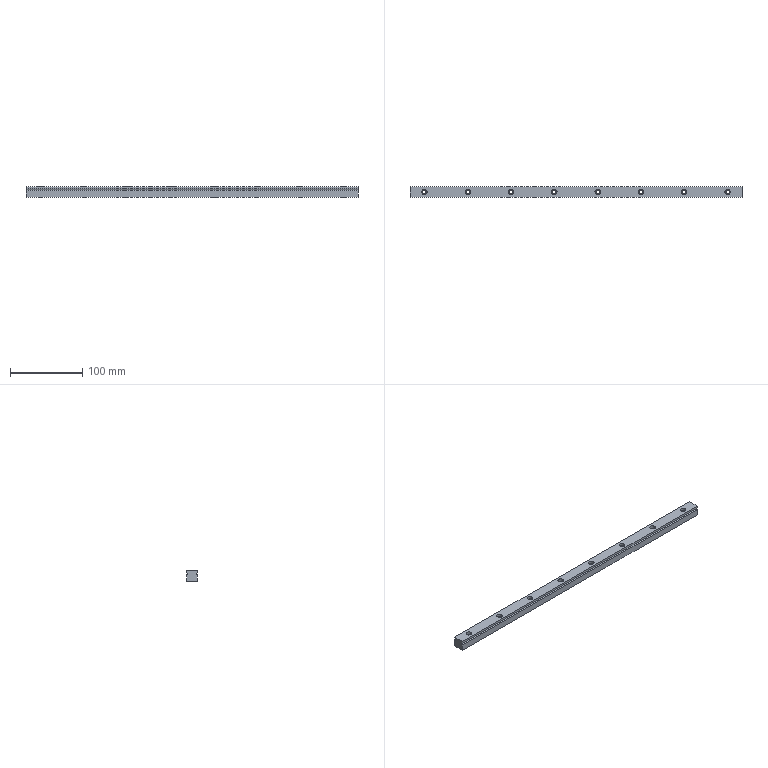Part | SolidWorks | features BaseBody 1 | 1 solid | 50 faces | box 460 x 15 x 15 mm | volume 98244 mm3 | cylinder 34 | plane 16 | commonest cylinder face diameters 4.5 x16 7.5 x16 2.6 x2
STEP:
#1=CARTESIAN_POINT('',(212.25,0.,0.));
#2=VERTEX_POINT('',#1);
#3=CARTESIAN_POINT('',(207.75,0.,0.));
#4=VERTEX_POINT('',#3);
#5=CARTESIAN_POINT('',(210.,0.,0.));
#6=DIRECTION('',(0.,0.,-1.));
#7=DIRECTION('',(1.,0.,0.));
#8=AXIS2_PLACEMENT_3D('',#5,#6,#7);
#9=CIRCLE('',#8,2.25);
#10=EDGE_CURVE('',#2,#4,#9,.T.);
#11=ORIENTED_EDGE('',*,*,#10,.T.);
#12=CARTESIAN_POINT('',(207.75,0.,11.));
#13=VERTEX_POINT('',#12);
#14=CARTESIAN_POINT('',(207.75,0.,-1.));
#15=DIRECTION('',(0.,0.,1.));
#16=VECTOR('',#15,1000.);
#17=LINE('',#14,#16);
#18=EDGE_CURVE('',#4,#13,#17,.T.);
#19=ORIENTED_EDGE('',*,*,#18,.T.);
#20=CARTESIAN_POINT('',(212.25,0.,11.));
#21=VERTEX_POINT('',#20);
#22=CARTESIAN_POINT('',(210.,0.,11.));
#23=DIRECTION('',(0.,0.,-1.));
#24=DIRECTION('',(1.,0.,0.));
#25=AXIS2_PLACEMENT_3D('',#22,#23,#24);
#26=CIRCLE('',#25,2.25);
#27=EDGE_CURVE('',#21,#13,#26,.T.);
#28=ORIENTED_EDGE('',*,*,#27,.F.);
#29=CARTESIAN_POINT('',(212.25,0.,-1.));
#30=DIRECTION('',(0.,0.,1.));
#31=VECTOR('',#30,1000.);
#32=LINE('',#29,#31);
#33=EDGE_CURVE('',#2,#21,#32,.T.);
#34=ORIENTED_EDGE('',*,*,#33,.F.);
#35=EDGE_LOOP('',(#11,#19,#28,#34));
#36=FACE_OUTER_BOUND('',#35,.T.);
#37=CARTESIAN_POINT('',(210.,0.,-1.));
#38=DIRECTION('',(0.,0.,1.));
#39=DIRECTION('',(1.,0.,0.));
#40=AXIS2_PLACEMENT_3D('',#37,#38,#39);
#41=CYLINDRICAL_SURFACE('',#40,2.25);
#42=ADVANCED_FACE('',(#36),#41,.F.);
#43=CARTESIAN_POINT('',(152.25,0.,0.));
#44=VERTEX_POINT('',#43);
#45=CARTESIAN_POINT('',(147.75,0.,0.));
#46=VERTEX_POINT('',#45);
#47=CARTESIAN_POINT('',(150.,0.,0.));
#48=DIRECTION('',(0.,0.,-1.));
#49=DIRECTION('',(1.,0.,0.));
#50=AXIS2_PLACEMENT_3D('',#47,#48,#49);
#51=CIRCLE('',#50,2.25);
#52=EDGE_CURVE('',#44,#46,#51,.T.);
#53=ORIENTED_EDGE('',*,*,#52,.T.);
#54=CARTESIAN_POINT('',(147.75,0.,11.));
#55=VERTEX_POINT('',#54);
#56=CARTESIAN_POINT('',(147.75,0.,-1.));
#57=DIRECTION('',(0.,0.,1.));
#58=VECTOR('',#57,1000.);
#59=LINE('',#56,#58);
#60=EDGE_CURVE('',#46,#55,#59,.T.);
#61=ORIENTED_EDGE('',*,*,#60,.T.);
#62=CARTESIAN_POINT('',(152.25,0.,11.));
#63=VERTEX_POINT('',#62);
#64=CARTESIAN_POINT('',(150.,0.,11.));
#65=DIRECTION('',(0.,0.,-1.));
#66=DIRECTION('',(1.,0.,0.));
#67=AXIS2_PLACEMENT_3D('',#64,#65,#66);
#68=CIRCLE('',#67,2.25);
#69=EDGE_CURVE('',#63,#55,#68,.T.);
#70=ORIENTED_EDGE('',*,*,#69,.F.);
#71=CARTESIAN_POINT('',(152.25,0.,-1.));
#72=DIRECTION('',(0.,0.,1.));
#73=VECTOR('',#72,1000.);
#74=LINE('',#71,#73);
#75=EDGE_CURVE('',#44,#63,#74,.T.);
#76=ORIENTED_EDGE('',*,*,#75,.F.);
#77=EDGE_LOOP('',(#53,#61,#70,#76));
#78=FACE_OUTER_BOUND('',#77,.T.);
#79=CARTESIAN_POINT('',(150.,0.,-1.));
#80=DIRECTION('',(0.,0.,1.));
#81=DIRECTION('',(1.,0.,0.));
#82=AXIS2_PLACEMENT_3D('',#79,#80,#81);
#83=CYLINDRICAL_SURFACE('',#82,2.25);
#84=ADVANCED_FACE('',(#78),#83,.F.);
#85=CARTESIAN_POINT('',(92.25,0.,0.));
#86=VERTEX_POINT('',#85);
#87=CARTESIAN_POINT('',(87.75,0.,0.));
#88=VERTEX_POINT('',#87);
#89=CARTESIAN_POINT('',(90.,0.,0.));
#90=DIRECTION('',(0.,0.,-1.));
#91=DIRECTION('',(1.,0.,0.));
#92=AXIS2_PLACEMENT_3D('',#89,#90,#91);
#93=CIRCLE('',#92,2.25);
#94=EDGE_CURVE('',#86,#88,#93,.T.);
#95=ORIENTED_EDGE('',*,*,#94,.T.);
#96=CARTESIAN_POINT('',(87.75,0.,11.));
#97=VERTEX_POINT('',#96);
#98=CARTESIAN_POINT('',(87.75,0.,-1.));
#99=DIRECTION('',(0.,0.,1.));
#100=VECTOR('',#99,1000.);
#101=LINE('',#98,#100);
#102=EDGE_CURVE('',#88,#97,#101,.T.);
#103=ORIENTED_EDGE('',*,*,#102,.T.);
#104=CARTESIAN_POINT('',(92.25,0.,11.));
#105=VERTEX_POINT('',#104);
#106=CARTESIAN_POINT('',(90.,0.,11.));
#107=DIRECTION('',(0.,0.,-1.));
#108=DIRECTION('',(1.,0.,0.));
#109=AXIS2_PLACEMENT_3D('',#106,#107,#108);
#110=CIRCLE('',#109,2.25);
#111=EDGE_CURVE('',#105,#97,#110,.T.);
#112=ORIENTED_EDGE('',*,*,#111,.F.);
#113=CARTESIAN_POINT('',(92.25,0.,-1.));
#114=DIRECTION('',(0.,0.,1.));
#115=VECTOR('',#114,1000.);
#116=LINE('',#113,#115);
#117=EDGE_CURVE('',#86,#105,#116,.T.);
#118=ORIENTED_EDGE('',*,*,#117,.F.);
#119=EDGE_LOOP('',(#95,#103,#112,#118));
#120=FACE_OUTER_BOUND('',#119,.T.);
#121=CARTESIAN_POINT('',(90.,0.,-1.));
#122=DIRECTION('',(0.,0.,1.));
#123=DIRECTION('',(1.,0.,0.));
#124=AXIS2_PLACEMENT_3D('',#121,#122,#123);
#125=CYLINDRICAL_SURFACE('',#124,2.25);
#126=ADVANCED_FACE('',(#120),#125,.F.);
#127=CARTESIAN_POINT('',(32.25,0.,0.));
#128=VERTEX_POINT('',#127);
#129=CARTESIAN_POINT('',(27.75,0.,0.));
#130=VERTEX_POINT('',#129);
#131=CARTESIAN_POINT('',(30.,0.,0.));
#132=DIRECTION('',(0.,0.,-1.));
#133=DIRECTION('',(1.,0.,0.));
#134=AXIS2_PLACEMENT_3D('',#131,#132,#133);
#135=CIRCLE('',#134,2.25);
#136=EDGE_CURVE('',#128,#130,#135,.T.);
#137=ORIENTED_EDGE('',*,*,#136,.T.);
#138=CARTESIAN_POINT('',(27.75,0.,11.));
#139=VERTEX_POINT('',#138);
#140=CARTESIAN_POINT('',(27.75,0.,-1.));
#141=DIRECTION('',(0.,0.,1.));
#142=VECTOR('',#141,1000.);
#143=LINE('',#140,#142);
#144=EDGE_CURVE('',#130,#139,#143,.T.);
#145=ORIENTED_EDGE('',*,*,#144,.T.);
#146=CARTESIAN_POINT('',(32.25,0.,11.));
#147=VERTEX_POINT('',#146);
#148=CARTESIAN_POINT('',(30.,0.,11.));
#149=DIRECTION('',(0.,0.,-1.));
#150=DIRECTION('',(1.,0.,0.));
#151=AXIS2_PLACEMENT_3D('',#148,#149,#150);
#152=CIRCLE('',#151,2.25);
#153=EDGE_CURVE('',#147,#139,#152,.T.);
#154=ORIENTED_EDGE('',*,*,#153,.F.);
#155=CARTESIAN_POINT('',(32.25,0.,-1.));
#156=DIRECTION('',(0.,0.,1.));
#157=VECTOR('',#156,1000.);
#158=LINE('',#155,#157);
#159=EDGE_CURVE('',#128,#147,#158,.T.);
#160=ORIENTED_EDGE('',*,*,#159,.F.);
#161=EDGE_LOOP('',(#137,#145,#154,#160));
#162=FACE_OUTER_BOUND('',#161,.T.);
#163=CARTESIAN_POINT('',(30.,0.,-1.));
#164=DIRECTION('',(0.,0.,1.));
#165=DIRECTION('',(1.,0.,0.));
#166=AXIS2_PLACEMENT_3D('',#163,#164,#165);
#167=CYLINDRICAL_SURFACE('',#166,2.25);
#168=ADVANCED_FACE('',(#162),#167,.F.);
#169=CARTESIAN_POINT('',(-27.75,0.,0.));
#170=VERTEX_POINT('',#169);
#171=CARTESIAN_POINT('',(-32.25,0.,0.));
#172=VERTEX_POINT('',#171);
#173=CARTESIAN_POINT('',(-30.,0.,0.));
#174=DIRECTION('',(0.,0.,-1.));
#175=DIRECTION('',(1.,0.,0.));
#176=AXIS2_PLACEMENT_3D('',#173,#174,#175);
#177=CIRCLE('',#176,2.25);
#178=EDGE_CURVE('',#170,#172,#177,.T.);
#179=ORIENTED_EDGE('',*,*,#178,.T.);
#180=CARTESIAN_POINT('',(-32.25,0.,11.));
#181=VERTEX_POINT('',#180);
#182=CARTESIAN_POINT('',(-32.25,0.,-1.));
#183=DIRECTION('',(0.,0.,1.));
#184=VECTOR('',#183,1000.);
#185=LINE('',#182,#184);
#186=EDGE_CURVE('',#172,#181,#185,.T.);
#187=ORIENTED_EDGE('',*,*,#186,.T.);
#188=CARTESIAN_POINT('',(-27.75,0.,11.));
#189=VERTEX_POINT('',#188);
#190=CARTESIAN_POINT('',(-30.,0.,11.));
#191=DIRECTION('',(0.,0.,-1.));
#192=DIRECTION('',(1.,0.,0.));
#193=AXIS2_PLACEMENT_3D('',#190,#191,#192);
#194=CIRCLE('',#193,2.25);
#195=EDGE_CURVE('',#189,#181,#194,.T.);
#196=ORIENTED_EDGE('',*,*,#195,.F.);
#197=CARTESIAN_POINT('',(-27.75,0.,-1.));
#198=DIRECTION('',(0.,0.,1.));
#199=VECTOR('',#198,1000.);
#200=LINE('',#197,#199);
#201=EDGE_CURVE('',#170,#189,#200,.T.);
#202=ORIENTED_EDGE('',*,*,#201,.F.);
#203=EDGE_LOOP('',(#179,#187,#196,#202));
#204=FACE_OUTER_BOUND('',#203,.T.);
#205=CARTESIAN_POINT('',(-30.,0.,-1.));
#206=DIRECTION('',(0.,0.,1.));
#207=DIRECTION('',(1.,0.,0.));
#208=AXIS2_PLACEMENT_3D('',#205,#206,#207);
#209=CYLINDRICAL_SURFACE('',#208,2.25);
#210=ADVANCED_FACE('',(#204),#209,.F.);
#211=CARTESIAN_POINT('',(-87.75,0.,0.));
#212=VERTEX_POINT('',#211);
#213=CARTESIAN_POINT('',(-92.25,0.,0.));
#214=VERTEX_POINT('',#213);
#215=CARTESIAN_POINT('',(-90.,0.,0.));
#216=DIRECTION('',(0.,0.,-1.));
#217=DIRECTION('',(1.,0.,0.));
#218=AXIS2_PLACEMENT_3D('',#215,#216,#217);
#219=CIRCLE('',#218,2.25);
#220=EDGE_CURVE('',#212,#214,#219,.T.);
#221=ORIENTED_EDGE('',*,*,#220,.T.);
#222=CARTESIAN_POINT('',(-92.25,0.,11.));
#223=VERTEX_POINT('',#222);
#224=CARTESIAN_POINT('',(-92.25,0.,-1.));
#225=DIRECTION('',(0.,0.,1.));
#226=VECTOR('',#225,1000.);
#227=LINE('',#224,#226);
#228=EDGE_CURVE('',#214,#223,#227,.T.);
#229=ORIENTED_EDGE('',*,*,#228,.T.);
#230=CARTESIAN_POINT('',(-87.75,0.,11.));
#231=VERTEX_POINT('',#230);
#232=CARTESIAN_POINT('',(-90.,0.,11.));
#233=DIRECTION('',(0.,0.,-1.));
#234=DIRECTION('',(1.,0.,0.));
#235=AXIS2_PLACEMENT_3D('',#232,#233,#234);
#236=CIRCLE('',#235,2.25);
#237=EDGE_CURVE('',#231,#223,#236,.T.);
#238=ORIENTED_EDGE('',*,*,#237,.F.);
#239=CARTESIAN_POINT('',(-87.75,0.,-1.));
#240=DIRECTION('',(0.,0.,1.));
#241=VECTOR('',#240,1000.);
#242=LINE('',#239,#241);
#243=EDGE_CURVE('',#212,#231,#242,.T.);
#244=ORIENTED_EDGE('',*,*,#243,.F.);
#245=EDGE_LOOP('',(#221,#229,#238,#244));
#246=FACE_OUTER_BOUND('',#245,.T.);
#247=CARTESIAN_POINT('',(-90.,0.,-1.));
#248=DIRECTION('',(0.,0.,1.));
#249=DIRECTION('',(1.,0.,0.));
#250=AXIS2_PLACEMENT_3D('',#247,#248,#249);
#251=CYLINDRICAL_SURFACE('',#250,2.25);
#252=ADVANCED_FACE('',(#246),#251,.F.);
#253=CARTESIAN_POINT('',(-147.75,0.,0.));
#254=VERTEX_POINT('',#253);
#255=CARTESIAN_POINT('',(-152.25,0.,0.));
#256=VERTEX_POINT('',#255);
#257=CARTESIAN_POINT('',(-150.,0.,0.));
#258=DIRECTION('',(0.,0.,-1.));
#259=DIRECTION('',(1.,0.,0.));
#260=AXIS2_PLACEMENT_3D('',#257,#258,#259);
#261=CIRCLE('',#260,2.25);
#262=EDGE_CURVE('',#254,#256,#261,.T.);
#263=ORIENTED_EDGE('',*,*,#262,.T.);
#264=CARTESIAN_POINT('',(-152.25,0.,11.));
#265=VERTEX_POINT('',#264);
#266=CARTESIAN_POINT('',(-152.25,0.,-1.));
#267=DIRECTION('',(0.,0.,1.));
#268=VECTOR('',#267,1000.);
#269=LINE('',#266,#268);
#270=EDGE_CURVE('',#256,#265,#269,.T.);
#271=ORIENTED_EDGE('',*,*,#270,.T.);
#272=CARTESIAN_POINT('',(-147.75,0.,11.));
#273=VERTEX_POINT('',#272);
#274=CARTESIAN_POINT('',(-150.,0.,11.));
#275=DIRECTION('',(0.,0.,-1.));
#276=DIRECTION('',(1.,0.,0.));
#277=AXIS2_PLACEMENT_3D('',#274,#275,#276);
#278=CIRCLE('',#277,2.25);
#279=EDGE_CURVE('',#273,#265,#278,.T.);
#280=ORIENTED_EDGE('',*,*,#279,.F.);
#281=CARTESIAN_POINT('',(-147.75,0.,-1.));
#282=DIRECTION('',(0.,0.,1.));
#283=VECTOR('',#282,1000.);
#284=LINE('',#281,#283);
#285=EDGE_CURVE('',#254,#273,#284,.T.);
#286=ORIENTED_EDGE('',*,*,#285,.F.);
#287=EDGE_LOOP('',(#263,#271,#280,#286));
#288=FACE_OUTER_BOUND('',#287,.T.);
#289=CARTESIAN_POINT('',(-150.,0.,-1.));
#290=DIRECTION('',(0.,0.,1.));
#291=DIRECTION('',(1.,0.,0.));
#292=AXIS2_PLACEMENT_3D('',#289,#290,#291);
#293=CYLINDRICAL_SURFACE('',#292,2.25);
#294=ADVANCED_FACE('',(#288),#293,.F.);
#295=CARTESIAN_POINT('',(-207.75,0.,0.));
#296=VERTEX_POINT('',#295);
#297=CARTESIAN_POINT('',(-212.25,0.,0.));
#298=VERTEX_POINT('',#297);
#299=CARTESIAN_POINT('',(-210.,0.,0.));
#300=DIRECTION('',(0.,0.,-1.));
#301=DIRECTION('',(1.,0.,0.));
#302=AXIS2_PLACEMENT_3D('',#299,#300,#301);
#303=CIRCLE('',#302,2.25);
#304=EDGE_CURVE('',#296,#298,#303,.T.);
#305=ORIENTED_EDGE('',*,*,#304,.T.);
#306=CARTESIAN_POINT('',(-212.25,0.,11.));
#307=VERTEX_POINT('',#306);
#308=CARTESIAN_POINT('',(-212.25,0.,-1.));
#309=DIRECTION('',(0.,0.,1.));
#310=VECTOR('',#309,1000.);
#311=LINE('',#308,#310);
#312=EDGE_CURVE('',#298,#307,#311,.T.);
#313=ORIENTED_EDGE('',*,*,#312,.T.);
#314=CARTESIAN_POINT('',(-207.75,0.,11.));
#315=VERTEX_POINT('',#314);
#316=CARTESIAN_POINT('',(-210.,0.,11.));
#317=DIRECTION('',(0.,0.,-1.));
#318=DIRECTION('',(1.,0.,0.));
#319=AXIS2_PLACEMENT_3D('',#316,#317,#318);
#320=CIRCLE('',#319,2.25);
#321=EDGE_CURVE('',#315,#307,#320,.T.);
#322=ORIENTED_EDGE('',*,*,#321,.F.);
#323=CARTESIAN_POINT('',(-207.75,0.,-1.));
#324=DIRECTION('',(0.,0.,1.));
#325=VECTOR('',#324,1000.);
#326=LINE('',#323,#325);
#327=EDGE_CURVE('',#296,#315,#326,.T.);
#328=ORIENTED_EDGE('',*,*,#327,.F.);
#329=EDGE_LOOP('',(#305,#313,#322,#328));
#330=FACE_OUTER_BOUND('',#329,.T.);
#331=CARTESIAN_POINT('',(-210.,0.,-1.));
#332=DIRECTION('',(0.,0.,1.));
#333=DIRECTION('',(1.,0.,0.));
#334=AXIS2_PLACEMENT_3D('',#331,#332,#333);
#335=CYLINDRICAL_SURFACE('',#334,2.25);
#336=ADVANCED_FACE('',(#330),#335,.F.);
#337=CARTESIAN_POINT('',(206.25,0.,11.));
#338=VERTEX_POINT('',#337);
#339=CARTESIAN_POINT('',(213.75,0.,11.));
#340=VERTEX_POINT('',#339);
#341=CARTESIAN_POINT('',(210.,0.,11.));
#342=DIRECTION('',(0.,0.,1.));
#343=DIRECTION('',(1.,0.,0.));
#344=AXIS2_PLACEMENT_3D('',#341,#342,#343);
#345=CIRCLE('',#344,3.75);
#346=EDGE_CURVE('',#338,#340,#345,.T.);
#347=ORIENTED_EDGE('',*,*,#346,.F.);
#348=CARTESIAN_POINT('',(206.25,0.,15.));
#349=VERTEX_POINT('',#348);
#350=CARTESIAN_POINT('',(206.25,0.,11.));
#351=DIRECTION('',(0.,0.,1.));
#352=VECTOR('',#351,1000.);
#353=LINE('',#350,#352);
#354=EDGE_CURVE('',#338,#349,#353,.T.);
#355=ORIENTED_EDGE('',*,*,#354,.T.);
#356=CARTESIAN_POINT('',(213.75,0.,15.));
#357=VERTEX_POINT('',#356);
#358=CARTESIAN_POINT('',(210.,0.,15.));
#359=DIRECTION('',(0.,0.,-1.));
#360=DIRECTION('',(1.,0.,0.));
#361=AXIS2_PLACEMENT_3D('',#358,#359,#360);
#362=CIRCLE('',#361,3.75);
#363=EDGE_CURVE('',#357,#349,#362,.T.);
#364=ORIENTED_EDGE('',*,*,#363,.F.);
#365=CARTESIAN_POINT('',(213.75,0.,11.));
#366=DIRECTION('',(0.,0.,1.));
#367=VECTOR('',#366,1000.);
#368=LINE('',#365,#367);
#369=EDGE_CURVE('',#340,#357,#368,.T.);
#370=ORIENTED_EDGE('',*,*,#369,.F.);
#371=EDGE_LOOP('',(#347,#355,#364,#370));
#372=FACE_OUTER_BOUND('',#371,.T.);
#373=CARTESIAN_POINT('',(210.,0.,11.));
#374=DIRECTION('',(0.,0.,1.));
#375=DIRECTION('',(1.,0.,0.));
#376=AXIS2_PLACEMENT_3D('',#373,#374,#375);
#377=CYLINDRICAL_SURFACE('',#376,3.75);
#378=ADVANCED_FACE('',(#372),#377,.F.);
#379=CARTESIAN_POINT('',(146.25,0.,11.));
#380=VERTEX_POINT('',#379);
#381=CARTESIAN_POINT('',(153.75,0.,11.));
#382=VERTEX_POINT('',#381);
#383=CARTESIAN_POINT('',(150.,0.,11.));
#384=DIRECTION('',(0.,0.,1.));
#385=DIRECTION('',(1.,0.,0.));
#386=AXIS2_PLACEMENT_3D('',#383,#384,#385);
#387=CIRCLE('',#386,3.75);
#388=EDGE_CURVE('',#380,#382,#387,.T.);
#389=ORIENTED_EDGE('',*,*,#388,.F.);
#390=CARTESIAN_POINT('',(146.25,0.,15.));
#391=VERTEX_POINT('',#390);
#392=CARTESIAN_POINT('',(146.25,0.,11.));
#393=DIRECTION('',(0.,0.,1.));
#394=VECTOR('',#393,1000.);
#395=LINE('',#392,#394);
#396=EDGE_CURVE('',#380,#391,#395,.T.);
#397=ORIENTED_EDGE('',*,*,#396,.T.);
#398=CARTESIAN_POINT('',(153.75,0.,15.));
#399=VERTEX_POINT('',#398);
#400=CARTESIAN_POINT('',(150.,0.,15.));
#401=DIRECTION('',(0.,0.,-1.));
#402=DIRECTION('',(1.,0.,0.));
#403=AXIS2_PLACEMENT_3D('',#400,#401,#402);
#404=CIRCLE('',#403,3.75);
#405=EDGE_CURVE('',#399,#391,#404,.T.);
#406=ORIENTED_EDGE('',*,*,#405,.F.);
#407=CARTESIAN_POINT('',(153.75,0.,11.));
#408=DIRECTION('',(0.,0.,1.));
#409=VECTOR('',#408,1000.);
#410=LINE('',#407,#409);
#411=EDGE_CURVE('',#382,#399,#410,.T.);
#412=ORIENTED_EDGE('',*,*,#411,.F.);
#413=EDGE_LOOP('',(#389,#397,#406,#412));
#414=FACE_OUTER_BOUND('',#413,.T.);
#415=CARTESIAN_POINT('',(150.,0.,11.));
#416=DIRECTION('',(0.,0.,1.));
#417=DIRECTION('',(1.,0.,0.));
#418=AXIS2_PLACEMENT_3D('',#415,#416,#417);
#419=CYLINDRICAL_SURFACE('',#418,3.75);
#420=ADVANCED_FACE('',(#414),#419,.F.);
#421=CARTESIAN_POINT('',(86.25,0.,11.));
#422=VERTEX_POINT('',#421);
#423=CARTESIAN_POINT('',(93.75,0.,11.));
#424=VERTEX_POINT('',#423);
#425=CARTESIAN_POINT('',(90.,0.,11.));
#426=DIRECTION('',(0.,0.,1.));
#427=DIRECTION('',(1.,0.,0.));
#428=AXIS2_PLACEMENT_3D('',#425,#426,#427);
#429=CIRCLE('',#428,3.75);
#430=EDGE_CURVE('',#422,#424,#429,.T.);
#431=ORIENTED_EDGE('',*,*,#430,.F.);
#432=CARTESIAN_POINT('',(86.25,0.,15.));
#433=VERTEX_POINT('',#432);
#434=CARTESIAN_POINT('',(86.25,0.,11.));
#435=DIRECTION('',(0.,0.,1.));
#436=VECTOR('',#435,1000.);
#437=LINE('',#434,#436);
#438=EDGE_CURVE('',#422,#433,#437,.T.);
#439=ORIENTED_EDGE('',*,*,#438,.T.);
#440=CARTESIAN_POINT('',(93.75,0.,15.));
#441=VERTEX_POINT('',#440);
#442=CARTESIAN_POINT('',(90.,0.,15.));
#443=DIRECTION('',(0.,0.,-1.));
#444=DIRECTION('',(1.,0.,0.));
#445=AXIS2_PLACEMENT_3D('',#442,#443,#444);
#446=CIRCLE('',#445,3.75);
#447=EDGE_CURVE('',#441,#433,#446,.T.);
#448=ORIENTED_EDGE('',*,*,#447,.F.);
#449=CARTESIAN_POINT('',(93.75,0.,11.));
#450=DIRECTION('',(0.,0.,1.));
#451=VECTOR('',#450,1000.);
#452=LINE('',#449,#451);
#453=EDGE_CURVE('',#424,#441,#452,.T.);
#454=ORIENTED_EDGE('',*,*,#453,.F.);
#455=EDGE_LOOP('',(#431,#439,#448,#454));
#456=FACE_OUTER_BOUND('',#455,.T.);
#457=CARTESIAN_POINT('',(90.,0.,11.));
#458=DIRECTION('',(0.,0.,1.));
#459=DIRECTION('',(1.,0.,0.));
#460=AXIS2_PLACEMENT_3D('',#457,#458,#459);
#461=CYLINDRICAL_SURFACE('',#460,3.75);
#462=ADVANCED_FACE('',(#456),#461,.F.);
#463=CARTESIAN_POINT('',(26.25,0.,11.));
#464=VERTEX_POINT('',#463);
#465=CARTESIAN_POINT('',(33.75,0.,11.));
#466=VERTEX_POINT('',#465);
#467=CARTESIAN_POINT('',(30.,0.,11.));
#468=DIRECTION('',(0.,0.,1.));
#469=DIRECTION('',(1.,0.,0.));
#470=AXIS2_PLACEMENT_3D('',#467,#468,#469);
#471=CIRCLE('',#470,3.75);
#472=EDGE_CURVE('',#464,#466,#471,.T.);
#473=ORIENTED_EDGE('',*,*,#472,.F.);
#474=CARTESIAN_POINT('',(26.25,0.,15.));
#475=VERTEX_POINT('',#474);
#476=CARTESIAN_POINT('',(26.25,0.,11.));
#477=DIRECTION('',(0.,0.,1.));
#478=VECTOR('',#477,1000.);
#479=LINE('',#476,#478);
#480=EDGE_CURVE('',#464,#475,#479,.T.);
#481=ORIENTED_EDGE('',*,*,#480,.T.);
#482=CARTESIAN_POINT('',(33.75,0.,15.));
#483=VERTEX_POINT('',#482);
#484=CARTESIAN_POINT('',(30.,0.,15.));
#485=DIRECTION('',(0.,0.,-1.));
#486=DIRECTION('',(1.,0.,0.));
#487=AXIS2_PLACEMENT_3D('',#484,#485,#486);
#488=CIRCLE('',#487,3.75);
#489=EDGE_CURVE('',#483,#475,#488,.T.);
#490=ORIENTED_EDGE('',*,*,#489,.F.);
#491=CARTESIAN_POINT('',(33.75,0.,11.));
#492=DIRECTION('',(0.,0.,1.));
#493=VECTOR('',#492,1000.);
#494=LINE('',#491,#493);
#495=EDGE_CURVE('',#466,#483,#494,.T.);
#496=ORIENTED_EDGE('',*,*,#495,.F.);
#497=EDGE_LOOP('',(#473,#481,#490,#496));
#498=FACE_OUTER_BOUND('',#497,.T.);
#499=CARTESIAN_POINT('',(30.,0.,11.));
#500=DIRECTION('',(0.,0.,1.));
#501=DIRECTION('',(1.,0.,0.));
#502=AXIS2_PLACEMENT_3D('',#499,#500,#501);
#503=CYLINDRICAL_SURFACE('',#502,3.75);
#504=ADVANCED_FACE('',(#498),#503,.F.);
#505=CARTESIAN_POINT('',(-33.75,0.,11.));
#506=VERTEX_POINT('',#505);
#507=CARTESIAN_POINT('',(-26.25,0.,11.));
#508=VERTEX_POINT('',#507);
#509=CARTESIAN_POINT('',(-30.,0.,11.));
#510=DIRECTION('',(0.,0.,1.));
#511=DIRECTION('',(1.,0.,0.));
#512=AXIS2_PLACEMENT_3D('',#509,#510,#511);
#513=CIRCLE('',#512,3.75);
#514=EDGE_CURVE('',#506,#508,#513,.T.);
#515=ORIENTED_EDGE('',*,*,#514,.F.);
#516=CARTESIAN_POINT('',(-33.75,0.,15.));
#517=VERTEX_POINT('',#516);
#518=CARTESIAN_POINT('',(-33.75,0.,11.));
#519=DIRECTION('',(0.,0.,1.));
#520=VECTOR('',#519,1000.);
#521=LINE('',#518,#520);
#522=EDGE_CURVE('',#506,#517,#521,.T.);
#523=ORIENTED_EDGE('',*,*,#522,.T.);
#524=CARTESIAN_POINT('',(-26.25,0.,15.));
#525=VERTEX_POINT('',#524);
#526=CARTESIAN_POINT('',(-30.,0.,15.));
#527=DIRECTION('',(0.,0.,-1.));
#528=DIRECTION('',(1.,0.,0.));
#529=AXIS2_PLACEMENT_3D('',#526,#527,#528);
#530=CIRCLE('',#529,3.75);
#531=EDGE_CURVE('',#525,#517,#530,.T.);
#532=ORIENTED_EDGE('',*,*,#531,.F.);
#533=CARTESIAN_POINT('',(-26.25,0.,11.));
#534=DIRECTION('',(0.,0.,1.));
#535=VECTOR('',#534,1000.);
#536=LINE('',#533,#535);
#537=EDGE_CURVE('',#508,#525,#536,.T.);
#538=ORIENTED_EDGE('',*,*,#537,.F.);
#539=EDGE_LOOP('',(#515,#523,#532,#538));
#540=FACE_OUTER_BOUND('',#539,.T.);
#541=CARTESIAN_POINT('',(-30.,0.,11.));
#542=DIRECTION('',(0.,0.,1.));
#543=DIRECTION('',(1.,0.,0.));
#544=AXIS2_PLACEMENT_3D('',#541,#542,#543);
#545=CYLINDRICAL_SURFACE('',#544,3.75);
#546=ADVANCED_FACE('',(#540),#545,.F.);
#547=CARTESIAN_POINT('',(-93.75,0.,11.));
#548=VERTEX_POINT('',#547);
#549=CARTESIAN_POINT('',(-86.25,0.,11.));
#550=VERTEX_POINT('',#549);
#551=CARTESIAN_POINT('',(-90.,0.,11.));
#552=DIRECTION('',(0.,0.,1.));
#553=DIRECTION('',(1.,0.,0.));
#554=AXIS2_PLACEMENT_3D('',#551,#552,#553);
#555=CIRCLE('',#554,3.75);
#556=EDGE_CURVE('',#548,#550,#555,.T.);
#557=ORIENTED_EDGE('',*,*,#556,.F.);
#558=CARTESIAN_POINT('',(-93.75,0.,15.));
#559=VERTEX_POINT('',#558);
#560=CARTESIAN_POINT('',(-93.75,0.,11.));
#561=DIRECTION('',(0.,0.,1.));
#562=VECTOR('',#561,1000.);
#563=LINE('',#560,#562);
#564=EDGE_CURVE('',#548,#559,#563,.T.);
#565=ORIENTED_EDGE('',*,*,#564,.T.);
#566=CARTESIAN_POINT('',(-86.25,0.,15.));
#567=VERTEX_POINT('',#566);
#568=CARTESIAN_POINT('',(-90.,0.,15.));
#569=DIRECTION('',(0.,0.,-1.));
#570=DIRECTION('',(1.,0.,0.));
#571=AXIS2_PLACEMENT_3D('',#568,#569,#570);
#572=CIRCLE('',#571,3.75);
#573=EDGE_CURVE('',#567,#559,#572,.T.);
#574=ORIENTED_EDGE('',*,*,#573,.F.);
#575=CARTESIAN_POINT('',(-86.25,0.,11.));
#576=DIRECTION('',(0.,0.,1.));
#577=VECTOR('',#576,1000.);
#578=LINE('',#575,#577);
#579=EDGE_CURVE('',#550,#567,#578,.T.);
#580=ORIENTED_EDGE('',*,*,#579,.F.);
#581=EDGE_LOOP('',(#557,#565,#574,#580));
#582=FACE_OUTER_BOUND('',#581,.T.);
#583=CARTESIAN_POINT('',(-90.,0.,11.));
#584=DIRECTION('',(0.,0.,1.));
#585=DIRECTION('',(1.,0.,0.));
#586=AXIS2_PLACEMENT_3D('',#583,#584,#585);
#587=CYLINDRICAL_SURFACE('',#586,3.75);
#588=ADVANCED_FACE('',(#582),#587,.F.);
#589=CARTESIAN_POINT('',(-153.75,0.,11.));
#590=VERTEX_POINT('',#589);
#591=CARTESIAN_POINT('',(-146.25,0.,11.));
#592=VERTEX_POINT('',#591);
#593=CARTESIAN_POINT('',(-150.,0.,11.));
#594=DIRECTION('',(0.,0.,1.));
#595=DIRECTION('',(1.,0.,0.));
#596=AXIS2_PLACEMENT_3D('',#593,#594,#595);
#597=CIRCLE('',#596,3.75);
#598=EDGE_CURVE('',#590,#592,#597,.T.);
#599=ORIENTED_EDGE('',*,*,#598,.F.);
#600=CARTESIAN_POINT('',(-153.75,0.,15.));
#601=VERTEX_POINT('',#600);
#602=CARTESIAN_POINT('',(-153.75,0.,11.));
#603=DIRECTION('',(0.,0.,1.));
#604=VECTOR('',#603,1000.);
#605=LINE('',#602,#604);
#606=EDGE_CURVE('',#590,#601,#605,.T.);
#607=ORIENTED_EDGE('',*,*,#606,.T.);
#608=CARTESIAN_POINT('',(-146.25,0.,15.));
#609=VERTEX_POINT('',#608);
#610=CARTESIAN_POINT('',(-150.,0.,15.));
#611=DIRECTION('',(0.,0.,-1.));
#612=DIRECTION('',(1.,0.,0.));
#613=AXIS2_PLACEMENT_3D('',#610,#611,#612);
#614=CIRCLE('',#613,3.75);
#615=EDGE_CURVE('',#609,#601,#614,.T.);
#616=ORIENTED_EDGE('',*,*,#615,.F.);
#617=CARTESIAN_POINT('',(-146.25,0.,11.));
#618=DIRECTION('',(0.,0.,1.));
#619=VECTOR('',#618,1000.);
#620=LINE('',#617,#619);
#621=EDGE_CURVE('',#592,#609,#620,.T.);
#622=ORIENTED_EDGE('',*,*,#621,.F.);
#623=EDGE_LOOP('',(#599,#607,#616,#622));
#624=FACE_OUTER_BOUND('',#623,.T.);
#625=CARTESIAN_POINT('',(-150.,0.,11.));
#626=DIRECTION('',(0.,0.,1.));
#627=DIRECTION('',(1.,0.,0.));
#628=AXIS2_PLACEMENT_3D('',#625,#626,#627);
#629=CYLINDRICAL_SURFACE('',#628,3.75);
#630=ADVANCED_FACE('',(#624),#629,.F.);
#631=CARTESIAN_POINT('',(-213.75,0.,11.));
#632=VERTEX_POINT('',#631);
#633=CARTESIAN_POINT('',(-206.25,0.,11.));
#634=VERTEX_POINT('',#633);
#635=CARTESIAN_POINT('',(-210.,0.,11.));
#636=DIRECTION('',(0.,0.,1.));
#637=DIRECTION('',(1.,0.,0.));
#638=AXIS2_PLACEMENT_3D('',#635,#636,#637);
#639=CIRCLE('',#638,3.75);
#640=EDGE_CURVE('',#632,#634,#639,.T.);
#641=ORIENTED_EDGE('',*,*,#640,.F.);
#642=CARTESIAN_POINT('',(-213.75,0.,15.));
#643=VERTEX_POINT('',#642);
#644=CARTESIAN_POINT('',(-213.75,0.,11.));
#645=DIRECTION('',(0.,0.,1.));
#646=VECTOR('',#645,1000.);
#647=LINE('',#644,#646);
#648=EDGE_CURVE('',#632,#643,#647,.T.);
#649=ORIENTED_EDGE('',*,*,#648,.T.);
#650=CARTESIAN_POINT('',(-206.25,0.,15.));
#651=VERTEX_POINT('',#650);
#652=CARTESIAN_POINT('',(-210.,0.,15.));
#653=DIRECTION('',(0.,0.,-1.));
#654=DIRECTION('',(1.,0.,0.));
#655=AXIS2_PLACEMENT_3D('',#652,#653,#654);
#656=CIRCLE('',#655,3.75);
#657=EDGE_CURVE('',#651,#643,#656,.T.);
#658=ORIENTED_EDGE('',*,*,#657,.F.);
#659=CARTESIAN_POINT('',(-206.25,0.,11.));
#660=DIRECTION('',(0.,0.,1.));
#661=VECTOR('',#660,1000.);
#662=LINE('',#659,#661);
#663=EDGE_CURVE('',#634,#651,#662,.T.);
#664=ORIENTED_EDGE('',*,*,#663,.F.);
#665=EDGE_LOOP('',(#641,#649,#658,#664));
#666=FACE_OUTER_BOUND('',#665,.T.);
#667=CARTESIAN_POINT('',(-210.,0.,11.));
#668=DIRECTION('',(0.,0.,1.));
#669=DIRECTION('',(1.,0.,0.));
#670=AXIS2_PLACEMENT_3D('',#667,#668,#669);
#671=CYLINDRICAL_SURFACE('',#670,3.75);
#672=ADVANCED_FACE('',(#666),#671,.F.);
#673=ORIENTED_EDGE('',*,*,#10,.F.);
#674=CARTESIAN_POINT('',(210.,0.,0.));
#675=DIRECTION('',(0.,0.,-1.));
#676=DIRECTION('',(1.,0.,0.));
#677=AXIS2_PLACEMENT_3D('',#674,#675,#676);
#678=CIRCLE('',#677,2.25);
#679=EDGE_CURVE('',#4,#2,#678,.T.);
#680=ORIENTED_EDGE('',*,*,#679,.F.);
#681=EDGE_LOOP('',(#673,#680));
#682=FACE_BOUND('',#681,.T.);
#683=ORIENTED_EDGE('',*,*,#52,.F.);
#684=CARTESIAN_POINT('',(150.,0.,0.));
#685=DIRECTION('',(0.,0.,-1.));
#686=DIRECTION('',(1.,0.,0.));
#687=AXIS2_PLACEMENT_3D('',#684,#685,#686);
#688=CIRCLE('',#687,2.25);
#689=EDGE_CURVE('',#46,#44,#688,.T.);
#690=ORIENTED_EDGE('',*,*,#689,.F.);
#691=EDGE_LOOP('',(#683,#690));
#692=FACE_BOUND('',#691,.T.);
#693=ORIENTED_EDGE('',*,*,#94,.F.);
#694=CARTESIAN_POINT('',(90.,0.,0.));
#695=DIRECTION('',(0.,0.,-1.));
#696=DIRECTION('',(1.,0.,0.));
#697=AXIS2_PLACEMENT_3D('',#694,#695,#696);
#698=CIRCLE('',#697,2.25);
#699=EDGE_CURVE('',#88,#86,#698,.T.);
#700=ORIENTED_EDGE('',*,*,#699,.F.);
#701=EDGE_LOOP('',(#693,#700));
#702=FACE_BOUND('',#701,.T.);
#703=ORIENTED_EDGE('',*,*,#136,.F.);
#704=CARTESIAN_POINT('',(30.,0.,0.));
#705=DIRECTION('',(0.,0.,-1.));
#706=DIRECTION('',(1.,0.,0.));
#707=AXIS2_PLACEMENT_3D('',#704,#705,#706);
#708=CIRCLE('',#707,2.25);
#709=EDGE_CURVE('',#130,#128,#708,.T.);
#710=ORIENTED_EDGE('',*,*,#709,.F.);
#711=EDGE_LOOP('',(#703,#710));
#712=FACE_BOUND('',#711,.T.);
#713=ORIENTED_EDGE('',*,*,#178,.F.);
#714=CARTESIAN_POINT('',(-30.,0.,0.));
#715=DIRECTION('',(0.,0.,-1.));
#716=DIRECTION('',(1.,0.,0.));
#717=AXIS2_PLACEMENT_3D('',#714,#715,#716);
#718=CIRCLE('',#717,2.25);
#719=EDGE_CURVE('',#172,#170,#718,.T.);
#720=ORIENTED_EDGE('',*,*,#719,.F.);
#721=EDGE_LOOP('',(#713,#720));
#722=FACE_BOUND('',#721,.T.);
#723=ORIENTED_EDGE('',*,*,#220,.F.);
#724=CARTESIAN_POINT('',(-90.,0.,0.));
#725=DIRECTION('',(0.,0.,-1.));
#726=DIRECTION('',(1.,0.,0.));
#727=AXIS2_PLACEMENT_3D('',#724,#725,#726);
#728=CIRCLE('',#727,2.25);
#729=EDGE_CURVE('',#214,#212,#728,.T.);
#730=ORIENTED_EDGE('',*,*,#729,.F.);
#731=EDGE_LOOP('',(#723,#730));
#732=FACE_BOUND('',#731,.T.);
#733=ORIENTED_EDGE('',*,*,#262,.F.);
#734=CARTESIAN_POINT('',(-150.,0.,0.));
#735=DIRECTION('',(0.,0.,-1.));
#736=DIRECTION('',(1.,0.,0.));
#737=AXIS2_PLACEMENT_3D('',#734,#735,#736);
#738=CIRCLE('',#737,2.25);
#739=EDGE_CURVE('',#256,#254,#738,.T.);
#740=ORIENTED_EDGE('',*,*,#739,.F.);
#741=EDGE_LOOP('',(#733,#740));
#742=FACE_BOUND('',#741,.T.);
#743=ORIENTED_EDGE('',*,*,#304,.F.);
#744=CARTESIAN_POINT('',(-210.,0.,0.));
#745=DIRECTION('',(0.,0.,-1.));
#746=DIRECTION('',(1.,0.,0.));
#747=AXIS2_PLACEMENT_3D('',#744,#745,#746);
#748=CIRCLE('',#747,2.25);
#749=EDGE_CURVE('',#298,#296,#748,.T.);
#750=ORIENTED_EDGE('',*,*,#749,.F.);
#751=EDGE_LOOP('',(#743,#750));
#752=FACE_BOUND('',#751,.T.);
#753=CARTESIAN_POINT('',(230.,-7.5,0.));
#754=VERTEX_POINT('',#753);
#755=CARTESIAN_POINT('',(230.,7.5,0.));
#756=VERTEX_POINT('',#755);
#757=CARTESIAN_POINT('',(230.,-7.5,0.));
#758=DIRECTION('',(0.,1.,0.));
#759=VECTOR('',#758,1000.);
#760=LINE('',#757,#759);
#761=EDGE_CURVE('',#754,#756,#760,.T.);
#762=ORIENTED_EDGE('',*,*,#761,.F.);
#763=CARTESIAN_POINT('',(-230.,-7.5,0.));
#764=VERTEX_POINT('',#763);
#765=CARTESIAN_POINT('',(-230.,-7.5,0.));
#766=DIRECTION('',(1.,0.,0.));
#767=VECTOR('',#766,1000.);
#768=LINE('',#765,#767);
#769=EDGE_CURVE('',#764,#754,#768,.T.);
#770=ORIENTED_EDGE('',*,*,#769,.F.);
#771=CARTESIAN_POINT('',(-230.,7.5,0.));
#772=VERTEX_POINT('',#771);
#773=CARTESIAN_POINT('',(-230.,-7.5,0.));
#774=DIRECTION('',(0.,-1.,0.));
#775=VECTOR('',#774,1000.);
#776=LINE('',#773,#775);
#777=EDGE_CURVE('',#772,#764,#776,.T.);
#778=ORIENTED_EDGE('',*,*,#777,.F.);
#779=CARTESIAN_POINT('',(-230.,7.5,0.));
#780=DIRECTION('',(-1.,0.,0.));
#781=VECTOR('',#780,1000.);
#782=LINE('',#779,#781);
#783=EDGE_CURVE('',#756,#772,#782,.T.);
#784=ORIENTED_EDGE('',*,*,#783,.F.);
#785=EDGE_LOOP('',(#762,#770,#778,#784));
#786=FACE_OUTER_BOUND('',#785,.T.);
#787=CARTESIAN_POINT('',(-230.,-7.5,0.));
#788=DIRECTION('',(0.,0.,1.));
#789=DIRECTION('',(1.,0.,0.));
#790=AXIS2_PLACEMENT_3D('',#787,#788,#789);
#791=PLANE('',#790);
#792=ADVANCED_FACE('',(#682,#692,#702,#712,#722,#732,#742,#752,#786),#791,.F.);
#793=ORIENTED_EDGE('',*,*,#18,.F.);
#794=ORIENTED_EDGE('',*,*,#679,.T.);
#795=ORIENTED_EDGE('',*,*,#33,.T.);
#796=CARTESIAN_POINT('',(210.,0.,11.));
#797=DIRECTION('',(0.,0.,-1.));
#798=DIRECTION('',(1.,0.,0.));
#799=AXIS2_PLACEMENT_3D('',#796,#797,#798);
#800=CIRCLE('',#799,2.25);
#801=EDGE_CURVE('',#13,#21,#800,.T.);
#802=ORIENTED_EDGE('',*,*,#801,.F.);
#803=EDGE_LOOP('',(#793,#794,#795,#802));
#804=FACE_OUTER_BOUND('',#803,.T.);
#805=CARTESIAN_POINT('',(210.,0.,-1.));
#806=DIRECTION('',(0.,0.,1.));
#807=DIRECTION('',(1.,0.,0.));
#808=AXIS2_PLACEMENT_3D('',#805,#806,#807);
#809=CYLINDRICAL_SURFACE('',#808,2.25);
#810=ADVANCED_FACE('',(#804),#809,.F.);
#811=ORIENTED_EDGE('',*,*,#60,.F.);
#812=ORIENTED_EDGE('',*,*,#689,.T.);
#813=ORIENTED_EDGE('',*,*,#75,.T.);
#814=CARTESIAN_POINT('',(150.,0.,11.));
#815=DIRECTION('',(0.,0.,-1.));
#816=DIRECTION('',(1.,0.,0.));
#817=AXIS2_PLACEMENT_3D('',#814,#815,#816);
#818=CIRCLE('',#817,2.25);
#819=EDGE_CURVE('',#55,#63,#818,.T.);
#820=ORIENTED_EDGE('',*,*,#819,.F.);
#821=EDGE_LOOP('',(#811,#812,#813,#820));
#822=FACE_OUTER_BOUND('',#821,.T.);
#823=CARTESIAN_POINT('',(150.,0.,-1.));
#824=DIRECTION('',(0.,0.,1.));
#825=DIRECTION('',(1.,0.,0.));
#826=AXIS2_PLACEMENT_3D('',#823,#824,#825);
#827=CYLINDRICAL_SURFACE('',#826,2.25);
#828=ADVANCED_FACE('',(#822),#827,.F.);
#829=ORIENTED_EDGE('',*,*,#102,.F.);
#830=ORIENTED_EDGE('',*,*,#699,.T.);
#831=ORIENTED_EDGE('',*,*,#117,.T.);
#832=CARTESIAN_POINT('',(90.,0.,11.));
#833=DIRECTION('',(0.,0.,-1.));
#834=DIRECTION('',(1.,0.,0.));
#835=AXIS2_PLACEMENT_3D('',#832,#833,#834);
#836=CIRCLE('',#835,2.25);
#837=EDGE_CURVE('',#97,#105,#836,.T.);
#838=ORIENTED_EDGE('',*,*,#837,.F.);
#839=EDGE_LOOP('',(#829,#830,#831,#838));
#840=FACE_OUTER_BOUND('',#839,.T.);
#841=CARTESIAN_POINT('',(90.,0.,-1.));
#842=DIRECTION('',(0.,0.,1.));
#843=DIRECTION('',(1.,0.,0.));
#844=AXIS2_PLACEMENT_3D('',#841,#842,#843);
#845=CYLINDRICAL_SURFACE('',#844,2.25);
#846=ADVANCED_FACE('',(#840),#845,.F.);
#847=ORIENTED_EDGE('',*,*,#144,.F.);
#848=ORIENTED_EDGE('',*,*,#709,.T.);
#849=ORIENTED_EDGE('',*,*,#159,.T.);
#850=CARTESIAN_POINT('',(30.,0.,11.));
#851=DIRECTION('',(0.,0.,-1.));
#852=DIRECTION('',(1.,0.,0.));
#853=AXIS2_PLACEMENT_3D('',#850,#851,#852);
#854=CIRCLE('',#853,2.25);
#855=EDGE_CURVE('',#139,#147,#854,.T.);
#856=ORIENTED_EDGE('',*,*,#855,.F.);
#857=EDGE_LOOP('',(#847,#848,#849,#856));
#858=FACE_OUTER_BOUND('',#857,.T.);
#859=CARTESIAN_POINT('',(30.,0.,-1.));
#860=DIRECTION('',(0.,0.,1.));
#861=DIRECTION('',(1.,0.,0.));
#862=AXIS2_PLACEMENT_3D('',#859,#860,#861);
#863=CYLINDRICAL_SURFACE('',#862,2.25);
#864=ADVANCED_FACE('',(#858),#863,.F.);
#865=ORIENTED_EDGE('',*,*,#186,.F.);
#866=ORIENTED_EDGE('',*,*,#719,.T.);
#867=ORIENTED_EDGE('',*,*,#201,.T.);
#868=CARTESIAN_POINT('',(-30.,0.,11.));
#869=DIRECTION('',(0.,0.,-1.));
#870=DIRECTION('',(1.,0.,0.));
#871=AXIS2_PLACEMENT_3D('',#868,#869,#870);
#872=CIRCLE('',#871,2.25);
#873=EDGE_CURVE('',#181,#189,#872,.T.);
#874=ORIENTED_EDGE('',*,*,#873,.F.);
#875=EDGE_LOOP('',(#865,#866,#867,#874));
#876=FACE_OUTER_BOUND('',#875,.T.);
#877=CARTESIAN_POINT('',(-30.,0.,-1.));
#878=DIRECTION('',(0.,0.,1.));
#879=DIRECTION('',(1.,0.,0.));
#880=AXIS2_PLACEMENT_3D('',#877,#878,#879);
#881=CYLINDRICAL_SURFACE('',#880,2.25);
#882=ADVANCED_FACE('',(#876),#881,.F.);
#883=ORIENTED_EDGE('',*,*,#228,.F.);
#884=ORIENTED_EDGE('',*,*,#729,.T.);
#885=ORIENTED_EDGE('',*,*,#243,.T.);
#886=CARTESIAN_POINT('',(-90.,0.,11.));
#887=DIRECTION('',(0.,0.,-1.));
#888=DIRECTION('',(1.,0.,0.));
#889=AXIS2_PLACEMENT_3D('',#886,#887,#888);
#890=CIRCLE('',#889,2.25);
#891=EDGE_CURVE('',#223,#231,#890,.T.);
#892=ORIENTED_EDGE('',*,*,#891,.F.);
#893=EDGE_LOOP('',(#883,#884,#885,#892));
#894=FACE_OUTER_BOUND('',#893,.T.);
#895=CARTESIAN_POINT('',(-90.,0.,-1.));
#896=DIRECTION('',(0.,0.,1.));
#897=DIRECTION('',(1.,0.,0.));
#898=AXIS2_PLACEMENT_3D('',#895,#896,#897);
#899=CYLINDRICAL_SURFACE('',#898,2.25);
#900=ADVANCED_FACE('',(#894),#899,.F.);
#901=ORIENTED_EDGE('',*,*,#270,.F.);
#902=ORIENTED_EDGE('',*,*,#739,.T.);
#903=ORIENTED_EDGE('',*,*,#285,.T.);
#904=CARTESIAN_POINT('',(-150.,0.,11.));
#905=DIRECTION('',(0.,0.,-1.));
#906=DIRECTION('',(1.,0.,0.));
#907=AXIS2_PLACEMENT_3D('',#904,#905,#906);
#908=CIRCLE('',#907,2.25);
#909=EDGE_CURVE('',#265,#273,#908,.T.);
#910=ORIENTED_EDGE('',*,*,#909,.F.);
#911=EDGE_LOOP('',(#901,#902,#903,#910));
#912=FACE_OUTER_BOUND('',#911,.T.);
#913=CARTESIAN_POINT('',(-150.,0.,-1.));
#914=DIRECTION('',(0.,0.,1.));
#915=DIRECTION('',(1.,0.,0.));
#916=AXIS2_PLACEMENT_3D('',#913,#914,#915);
#917=CYLINDRICAL_SURFACE('',#916,2.25);
#918=ADVANCED_FACE('',(#912),#917,.F.);
#919=ORIENTED_EDGE('',*,*,#312,.F.);
#920=ORIENTED_EDGE('',*,*,#749,.T.);
#921=ORIENTED_EDGE('',*,*,#327,.T.);
#922=CARTESIAN_POINT('',(-210.,0.,11.));
#923=DIRECTION('',(0.,0.,-1.));
#924=DIRECTION('',(1.,0.,0.));
#925=AXIS2_PLACEMENT_3D('',#922,#923,#924);
#926=CIRCLE('',#925,2.25);
#927=EDGE_CURVE('',#307,#315,#926,.T.);
#928=ORIENTED_EDGE('',*,*,#927,.F.);
#929=EDGE_LOOP('',(#919,#920,#921,#928));
#930=FACE_OUTER_BOUND('',#929,.T.);
#931=CARTESIAN_POINT('',(-210.,0.,-1.));
#932=DIRECTION('',(0.,0.,1.));
#933=DIRECTION('',(1.,0.,0.));
#934=AXIS2_PLACEMENT_3D('',#931,#932,#933);
#935=CYLINDRICAL_SURFACE('',#934,2.25);
#936=ADVANCED_FACE('',(#930),#935,.F.);
#937=CARTESIAN_POINT('',(-230.,7.5,9.2));
#938=VERTEX_POINT('',#937);
#939=CARTESIAN_POINT('',(-230.,7.5,0.));
#940=DIRECTION('',(0.,0.,1.));
#941=VECTOR('',#940,1000.);
#942=LINE('',#939,#941);
#943=EDGE_CURVE('',#772,#938,#942,.T.);
#944=ORIENTED_EDGE('',*,*,#943,.T.);
#945=CARTESIAN_POINT('',(230.,7.5,9.2));
#946=VERTEX_POINT('',#945);
#947=CARTESIAN_POINT('',(-230.,7.5,9.2));
#948=DIRECTION('',(1.,0.,0.));
#949=VECTOR('',#948,1000.);
#950=LINE('',#947,#949);
#951=EDGE_CURVE('',#938,#946,#950,.T.);
#952=ORIENTED_EDGE('',*,*,#951,.T.);
#953=CARTESIAN_POINT('',(230.,7.5,0.));
#954=DIRECTION('',(0.,0.,-1.));
#955=VECTOR('',#954,1000.);
#956=LINE('',#953,#955);
#957=EDGE_CURVE('',#946,#756,#956,.T.);
#958=ORIENTED_EDGE('',*,*,#957,.T.);
#959=ORIENTED_EDGE('',*,*,#783,.T.);
#960=EDGE_LOOP('',(#944,#952,#958,#959));
#961=FACE_OUTER_BOUND('',#960,.T.);
#962=CARTESIAN_POINT('',(-230.,7.5,0.));
#963=DIRECTION('',(0.,1.,0.));
#964=DIRECTION('',(0.,0.,1.));
#965=AXIS2_PLACEMENT_3D('',#962,#963,#964);
#966=PLANE('',#965);
#967=ADVANCED_FACE('',(#961),#966,.T.);
#968=CARTESIAN_POINT('',(230.,-7.5,15.));
#969=VERTEX_POINT('',#968);
#970=CARTESIAN_POINT('',(230.,-7.5,11.8));
#971=VERTEX_POINT('',#970);
#972=CARTESIAN_POINT('',(230.,-7.5,0.));
#973=DIRECTION('',(0.,0.,-1.));
#974=VECTOR('',#973,1000.);
#975=LINE('',#972,#974);
#976=EDGE_CURVE('',#969,#971,#975,.T.);
#977=ORIENTED_EDGE('',*,*,#976,.T.);
#978=CARTESIAN_POINT('',(230.,-7.5,9.2));
#979=VERTEX_POINT('',#978);
#980=CARTESIAN_POINT('',(230.,-7.5,10.5));
#981=DIRECTION('',(-1.,0.,0.));
#982=DIRECTION('',(0.,0.,-1.));
#983=AXIS2_PLACEMENT_3D('',#980,#981,#982);
#984=CIRCLE('',#983,1.3);
#985=EDGE_CURVE('',#971,#979,#984,.T.);
#986=ORIENTED_EDGE('',*,*,#985,.T.);
#987=CARTESIAN_POINT('',(230.,-7.5,0.));
#988=DIRECTION('',(0.,0.,-1.));
#989=VECTOR('',#988,1000.);
#990=LINE('',#987,#989);
#991=EDGE_CURVE('',#979,#754,#990,.T.);
#992=ORIENTED_EDGE('',*,*,#991,.T.);
#993=ORIENTED_EDGE('',*,*,#761,.T.);
#994=ORIENTED_EDGE('',*,*,#957,.F.);
#995=CARTESIAN_POINT('',(230.,7.5,11.8));
#996=VERTEX_POINT('',#995);
#997=CARTESIAN_POINT('',(230.,7.5,10.5));
#998=DIRECTION('',(-1.,0.,0.));
#999=DIRECTION('',(0.,0.,-1.));
#1000=AXIS2_PLACEMENT_3D('',#997,#998,#999);
#1001=CIRCLE('',#1000,1.3);
#1002=EDGE_CURVE('',#946,#996,#1001,.T.);
#1003=ORIENTED_EDGE('',*,*,#1002,.T.);
#1004=CARTESIAN_POINT('',(230.,7.5,15.));
#1005=VERTEX_POINT('',#1004);
#1006=CARTESIAN_POINT('',(230.,7.5,0.));
#1007=DIRECTION('',(0.,0.,1.));
#1008=VECTOR('',#1007,1000.);
#1009=LINE('',#1006,#1008);
#1010=EDGE_CURVE('',#996,#1005,#1009,.T.);
#1011=ORIENTED_EDGE('',*,*,#1010,.T.);
#1012=CARTESIAN_POINT('',(230.,-7.5,15.));
#1013=DIRECTION('',(0.,-1.,0.));
#1014=VECTOR('',#1013,1000.);
#1015=LINE('',#1012,#1014);
#1016=EDGE_CURVE('',#1005,#969,#1015,.T.);
#1017=ORIENTED_EDGE('',*,*,#1016,.T.);
#1018=EDGE_LOOP('',(#977,#986,#992,#993,#994,#1003,#1011,#1017));
#1019=FACE_OUTER_BOUND('',#1018,.T.);
#1020=CARTESIAN_POINT('',(230.,-7.5,0.));
#1021=DIRECTION('',(1.,0.,0.));
#1022=DIRECTION('',(0.,0.,-1.));
#1023=AXIS2_PLACEMENT_3D('',#1020,#1021,#1022);
#1024=PLANE('',#1023);
#1025=ADVANCED_FACE('',(#1019),#1024,.T.);
#1026=CARTESIAN_POINT('',(-230.,-7.5,9.2));
#1027=VERTEX_POINT('',#1026);
#1028=CARTESIAN_POINT('',(-230.,-7.5,0.));
#1029=DIRECTION('',(0.,0.,1.));
#1030=VECTOR('',#1029,1000.);
#1031=LINE('',#1028,#1030);
#1032=EDGE_CURVE('',#764,#1027,#1031,.T.);
#1033=ORIENTED_EDGE('',*,*,#1032,.F.);
#1034=ORIENTED_EDGE('',*,*,#769,.T.);
#1035=ORIENTED_EDGE('',*,*,#991,.F.);
#1036=CARTESIAN_POINT('',(-230.,-7.5,9.2));
#1037=DIRECTION('',(1.,0.,0.));
#1038=VECTOR('',#1037,1000.);
#1039=LINE('',#1036,#1038);
#1040=EDGE_CURVE('',#1027,#979,#1039,.T.);
#1041=ORIENTED_EDGE('',*,*,#1040,.F.);
#1042=EDGE_LOOP('',(#1033,#1034,#1035,#1041));
#1043=FACE_OUTER_BOUND('',#1042,.T.);
#1044=CARTESIAN_POINT('',(-230.,-7.5,0.));
#1045=DIRECTION('',(0.,1.,0.));
#1046=DIRECTION('',(0.,0.,1.));
#1047=AXIS2_PLACEMENT_3D('',#1044,#1045,#1046);
#1048=PLANE('',#1047);
#1049=ADVANCED_FACE('',(#1043),#1048,.F.);
#1050=CARTESIAN_POINT('',(-230.,-7.5,15.));
#1051=VERTEX_POINT('',#1050);
#1052=CARTESIAN_POINT('',(-230.,-7.5,11.8));
#1053=VERTEX_POINT('',#1052);
#1054=CARTESIAN_POINT('',(-230.,-7.5,0.));
#1055=DIRECTION('',(0.,0.,-1.));
#1056=VECTOR('',#1055,1000.);
#1057=LINE('',#1054,#1056);
#1058=EDGE_CURVE('',#1051,#1053,#1057,.T.);
#1059=ORIENTED_EDGE('',*,*,#1058,.F.);
#1060=CARTESIAN_POINT('',(-230.,7.5,15.));
#1061=VERTEX_POINT('',#1060);
#1062=CARTESIAN_POINT('',(-230.,-7.5,15.));
#1063=DIRECTION('',(0.,-1.,0.));
#1064=VECTOR('',#1063,1000.);
#1065=LINE('',#1062,#1064);
#1066=EDGE_CURVE('',#1061,#1051,#1065,.T.);
#1067=ORIENTED_EDGE('',*,*,#1066,.F.);
#1068=CARTESIAN_POINT('',(-230.,7.5,11.8));
#1069=VERTEX_POINT('',#1068);
#1070=CARTESIAN_POINT('',(-230.,7.5,0.));
#1071=DIRECTION('',(0.,0.,1.));
#1072=VECTOR('',#1071,1000.);
#1073=LINE('',#1070,#1072);
#1074=EDGE_CURVE('',#1069,#1061,#1073,.T.);
#1075=ORIENTED_EDGE('',*,*,#1074,.F.);
#1076=CARTESIAN_POINT('',(-230.,7.5,10.5));
#1077=DIRECTION('',(-1.,0.,0.));
#1078=DIRECTION('',(0.,0.,-1.));
#1079=AXIS2_PLACEMENT_3D('',#1076,#1077,#1078);
#1080=CIRCLE('',#1079,1.3);
#1081=EDGE_CURVE('',#938,#1069,#1080,.T.);
#1082=ORIENTED_EDGE('',*,*,#1081,.F.);
#1083=ORIENTED_EDGE('',*,*,#943,.F.);
#1084=ORIENTED_EDGE('',*,*,#777,.T.);
#1085=ORIENTED_EDGE('',*,*,#1032,.T.);
#1086=CARTESIAN_POINT('',(-230.,-7.5,10.5));
#1087=DIRECTION('',(-1.,0.,0.));
#1088=DIRECTION('',(0.,0.,-1.));
#1089=AXIS2_PLACEMENT_3D('',#1086,#1087,#1088);
#1090=CIRCLE('',#1089,1.3);
#1091=EDGE_CURVE('',#1053,#1027,#1090,.T.);
#1092=ORIENTED_EDGE('',*,*,#1091,.F.);
#1093=EDGE_LOOP('',(#1059,#1067,#1075,#1082,#1083,#1084,#1085,#1092));
#1094=FACE_OUTER_BOUND('',#1093,.T.);
#1095=CARTESIAN_POINT('',(-230.,-7.5,0.));
#1096=DIRECTION('',(1.,0.,0.));
#1097=DIRECTION('',(0.,0.,-1.));
#1098=AXIS2_PLACEMENT_3D('',#1095,#1096,#1097);
#1099=PLANE('',#1098);
#1100=ADVANCED_FACE('',(#1094),#1099,.F.);
#1101=ORIENTED_EDGE('',*,*,#27,.T.);
#1102=ORIENTED_EDGE('',*,*,#801,.T.);
#1103=EDGE_LOOP('',(#1101,#1102));
#1104=FACE_BOUND('',#1103,.T.);
#1105=CARTESIAN_POINT('',(210.,0.,11.));
#1106=DIRECTION('',(0.,0.,1.));
#1107=DIRECTION('',(1.,0.,0.));
#1108=AXIS2_PLACEMENT_3D('',#1105,#1106,#1107);
#1109=CIRCLE('',#1108,3.75);
#1110=EDGE_CURVE('',#340,#338,#1109,.T.);
#1111=ORIENTED_EDGE('',*,*,#1110,.T.);
#1112=ORIENTED_EDGE('',*,*,#346,.T.);
#1113=EDGE_LOOP('',(#1111,#1112));
#1114=FACE_OUTER_BOUND('',#1113,.T.);
#1115=CARTESIAN_POINT('',(210.,0.,11.));
#1116=DIRECTION('',(0.,0.,1.));
#1117=DIRECTION('',(1.,0.,0.));
#1118=AXIS2_PLACEMENT_3D('',#1115,#1116,#1117);
#1119=PLANE('',#1118);
#1120=ADVANCED_FACE('',(#1104,#1114),#1119,.T.);
#1121=ORIENTED_EDGE('',*,*,#69,.T.);
#1122=ORIENTED_EDGE('',*,*,#819,.T.);
#1123=EDGE_LOOP('',(#1121,#1122));
#1124=FACE_BOUND('',#1123,.T.);
#1125=CARTESIAN_POINT('',(150.,0.,11.));
#1126=DIRECTION('',(0.,0.,1.));
#1127=DIRECTION('',(1.,0.,0.));
#1128=AXIS2_PLACEMENT_3D('',#1125,#1126,#1127);
#1129=CIRCLE('',#1128,3.75);
#1130=EDGE_CURVE('',#382,#380,#1129,.T.);
#1131=ORIENTED_EDGE('',*,*,#1130,.T.);
#1132=ORIENTED_EDGE('',*,*,#388,.T.);
#1133=EDGE_LOOP('',(#1131,#1132));
#1134=FACE_OUTER_BOUND('',#1133,.T.);
#1135=CARTESIAN_POINT('',(150.,0.,11.));
#1136=DIRECTION('',(0.,0.,1.));
#1137=DIRECTION('',(1.,0.,0.));
#1138=AXIS2_PLACEMENT_3D('',#1135,#1136,#1137);
#1139=PLANE('',#1138);
#1140=ADVANCED_FACE('',(#1124,#1134),#1139,.T.);
#1141=ORIENTED_EDGE('',*,*,#111,.T.);
#1142=ORIENTED_EDGE('',*,*,#837,.T.);
#1143=EDGE_LOOP('',(#1141,#1142));
#1144=FACE_BOUND('',#1143,.T.);
#1145=CARTESIAN_POINT('',(90.,0.,11.));
#1146=DIRECTION('',(0.,0.,1.));
#1147=DIRECTION('',(1.,0.,0.));
#1148=AXIS2_PLACEMENT_3D('',#1145,#1146,#1147);
#1149=CIRCLE('',#1148,3.75);
#1150=EDGE_CURVE('',#424,#422,#1149,.T.);
#1151=ORIENTED_EDGE('',*,*,#1150,.T.);
#1152=ORIENTED_EDGE('',*,*,#430,.T.);
#1153=EDGE_LOOP('',(#1151,#1152));
#1154=FACE_OUTER_BOUND('',#1153,.T.);
#1155=CARTESIAN_POINT('',(90.,0.,11.));
#1156=DIRECTION('',(0.,0.,1.));
#1157=DIRECTION('',(1.,0.,0.));
#1158=AXIS2_PLACEMENT_3D('',#1155,#1156,#1157);
#1159=PLANE('',#1158);
#1160=ADVANCED_FACE('',(#1144,#1154),#1159,.T.);
#1161=ORIENTED_EDGE('',*,*,#153,.T.);
#1162=ORIENTED_EDGE('',*,*,#855,.T.);
#1163=EDGE_LOOP('',(#1161,#1162));
#1164=FACE_BOUND('',#1163,.T.);
#1165=CARTESIAN_POINT('',(30.,0.,11.));
#1166=DIRECTION('',(0.,0.,1.));
#1167=DIRECTION('',(1.,0.,0.));
#1168=AXIS2_PLACEMENT_3D('',#1165,#1166,#1167);
#1169=CIRCLE('',#1168,3.75);
#1170=EDGE_CURVE('',#466,#464,#1169,.T.);
#1171=ORIENTED_EDGE('',*,*,#1170,.T.);
#1172=ORIENTED_EDGE('',*,*,#472,.T.);
#1173=EDGE_LOOP('',(#1171,#1172));
#1174=FACE_OUTER_BOUND('',#1173,.T.);
#1175=CARTESIAN_POINT('',(30.,0.,11.));
#1176=DIRECTION('',(0.,0.,1.));
#1177=DIRECTION('',(1.,0.,0.));
#1178=AXIS2_PLACEMENT_3D('',#1175,#1176,#1177);
#1179=PLANE('',#1178);
#1180=ADVANCED_FACE('',(#1164,#1174),#1179,.T.);
#1181=ORIENTED_EDGE('',*,*,#195,.T.);
#1182=ORIENTED_EDGE('',*,*,#873,.T.);
#1183=EDGE_LOOP('',(#1181,#1182));
#1184=FACE_BOUND('',#1183,.T.);
#1185=CARTESIAN_POINT('',(-30.,0.,11.));
#1186=DIRECTION('',(0.,0.,1.));
#1187=DIRECTION('',(1.,0.,0.));
#1188=AXIS2_PLACEMENT_3D('',#1185,#1186,#1187);
#1189=CIRCLE('',#1188,3.75);
#1190=EDGE_CURVE('',#508,#506,#1189,.T.);
#1191=ORIENTED_EDGE('',*,*,#1190,.T.);
#1192=ORIENTED_EDGE('',*,*,#514,.T.);
#1193=EDGE_LOOP('',(#1191,#1192));
#1194=FACE_OUTER_BOUND('',#1193,.T.);
#1195=CARTESIAN_POINT('',(-30.,0.,11.));
#1196=DIRECTION('',(0.,0.,1.));
#1197=DIRECTION('',(1.,0.,0.));
#1198=AXIS2_PLACEMENT_3D('',#1195,#1196,#1197);
#1199=PLANE('',#1198);
#1200=ADVANCED_FACE('',(#1184,#1194),#1199,.T.);
#1201=ORIENTED_EDGE('',*,*,#237,.T.);
#1202=ORIENTED_EDGE('',*,*,#891,.T.);
#1203=EDGE_LOOP('',(#1201,#1202));
#1204=FACE_BOUND('',#1203,.T.);
#1205=CARTESIAN_POINT('',(-90.,0.,11.));
#1206=DIRECTION('',(0.,0.,1.));
#1207=DIRECTION('',(1.,0.,0.));
#1208=AXIS2_PLACEMENT_3D('',#1205,#1206,#1207);
#1209=CIRCLE('',#1208,3.75);
#1210=EDGE_CURVE('',#550,#548,#1209,.T.);
#1211=ORIENTED_EDGE('',*,*,#1210,.T.);
#1212=ORIENTED_EDGE('',*,*,#556,.T.);
#1213=EDGE_LOOP('',(#1211,#1212));
#1214=FACE_OUTER_BOUND('',#1213,.T.);
#1215=CARTESIAN_POINT('',(-90.,0.,11.));
#1216=DIRECTION('',(0.,0.,1.));
#1217=DIRECTION('',(1.,0.,0.));
#1218=AXIS2_PLACEMENT_3D('',#1215,#1216,#1217);
#1219=PLANE('',#1218);
#1220=ADVANCED_FACE('',(#1204,#1214),#1219,.T.);
#1221=ORIENTED_EDGE('',*,*,#279,.T.);
#1222=ORIENTED_EDGE('',*,*,#909,.T.);
#1223=EDGE_LOOP('',(#1221,#1222));
#1224=FACE_BOUND('',#1223,.T.);
#1225=CARTESIAN_POINT('',(-150.,0.,11.));
#1226=DIRECTION('',(0.,0.,1.));
#1227=DIRECTION('',(1.,0.,0.));
#1228=AXIS2_PLACEMENT_3D('',#1225,#1226,#1227);
#1229=CIRCLE('',#1228,3.75);
#1230=EDGE_CURVE('',#592,#590,#1229,.T.);
#1231=ORIENTED_EDGE('',*,*,#1230,.T.);
#1232=ORIENTED_EDGE('',*,*,#598,.T.);
#1233=EDGE_LOOP('',(#1231,#1232));
#1234=FACE_OUTER_BOUND('',#1233,.T.);
#1235=CARTESIAN_POINT('',(-150.,0.,11.));
#1236=DIRECTION('',(0.,0.,1.));
#1237=DIRECTION('',(1.,0.,0.));
#1238=AXIS2_PLACEMENT_3D('',#1235,#1236,#1237);
#1239=PLANE('',#1238);
#1240=ADVANCED_FACE('',(#1224,#1234),#1239,.T.);
#1241=ORIENTED_EDGE('',*,*,#321,.T.);
#1242=ORIENTED_EDGE('',*,*,#927,.T.);
#1243=EDGE_LOOP('',(#1241,#1242));
#1244=FACE_BOUND('',#1243,.T.);
#1245=CARTESIAN_POINT('',(-210.,0.,11.));
#1246=DIRECTION('',(0.,0.,1.));
#1247=DIRECTION('',(1.,0.,0.));
#1248=AXIS2_PLACEMENT_3D('',#1245,#1246,#1247);
#1249=CIRCLE('',#1248,3.75);
#1250=EDGE_CURVE('',#634,#632,#1249,.T.);
#1251=ORIENTED_EDGE('',*,*,#1250,.T.);
#1252=ORIENTED_EDGE('',*,*,#640,.T.);
#1253=EDGE_LOOP('',(#1251,#1252));
#1254=FACE_OUTER_BOUND('',#1253,.T.);
#1255=CARTESIAN_POINT('',(-210.,0.,11.));
#1256=DIRECTION('',(0.,0.,1.));
#1257=DIRECTION('',(1.,0.,0.));
#1258=AXIS2_PLACEMENT_3D('',#1255,#1256,#1257);
#1259=PLANE('',#1258);
#1260=ADVANCED_FACE('',(#1244,#1254),#1259,.T.);
#1261=CARTESIAN_POINT('',(-231.,7.5,11.8));
#1262=DIRECTION('',(-1.,0.,0.));
#1263=VECTOR('',#1262,1000.);
#1264=LINE('',#1261,#1263);
#1265=EDGE_CURVE('',#996,#1069,#1264,.T.);
#1266=ORIENTED_EDGE('',*,*,#1265,.F.);
#1267=ORIENTED_EDGE('',*,*,#1002,.F.);
#1268=ORIENTED_EDGE('',*,*,#951,.F.);
#1269=ORIENTED_EDGE('',*,*,#1081,.T.);
#1270=EDGE_LOOP('',(#1266,#1267,#1268,#1269));
#1271=FACE_OUTER_BOUND('',#1270,.T.);
#1272=CARTESIAN_POINT('',(-231.,7.5,10.5));
#1273=DIRECTION('',(1.,0.,0.));
#1274=DIRECTION('',(0.,0.,-1.));
#1275=AXIS2_PLACEMENT_3D('',#1272,#1273,#1274);
#1276=CYLINDRICAL_SURFACE('',#1275,1.3);
#1277=ADVANCED_FACE('',(#1271),#1276,.F.);
#1278=ORIENTED_EDGE('',*,*,#1091,.T.);
#1279=ORIENTED_EDGE('',*,*,#1040,.T.);
#1280=ORIENTED_EDGE('',*,*,#985,.F.);
#1281=CARTESIAN_POINT('',(-231.,-7.5,11.8));
#1282=DIRECTION('',(1.,0.,0.));
#1283=VECTOR('',#1282,1000.);
#1284=LINE('',#1281,#1283);
#1285=EDGE_CURVE('',#1053,#971,#1284,.T.);
#1286=ORIENTED_EDGE('',*,*,#1285,.F.);
#1287=EDGE_LOOP('',(#1278,#1279,#1280,#1286));
#1288=FACE_OUTER_BOUND('',#1287,.T.);
#1289=CARTESIAN_POINT('',(-231.,-7.5,10.5));
#1290=DIRECTION('',(1.,0.,0.));
#1291=DIRECTION('',(0.,0.,-1.));
#1292=AXIS2_PLACEMENT_3D('',#1289,#1290,#1291);
#1293=CYLINDRICAL_SURFACE('',#1292,1.3);
#1294=ADVANCED_FACE('',(#1288),#1293,.F.);
#1295=ORIENTED_EDGE('',*,*,#1058,.T.);
#1296=ORIENTED_EDGE('',*,*,#1285,.T.);
#1297=ORIENTED_EDGE('',*,*,#976,.F.);
#1298=CARTESIAN_POINT('',(-230.,-7.5,15.));
#1299=DIRECTION('',(1.,0.,0.));
#1300=VECTOR('',#1299,1000.);
#1301=LINE('',#1298,#1300);
#1302=EDGE_CURVE('',#1051,#969,#1301,.T.);
#1303=ORIENTED_EDGE('',*,*,#1302,.F.);
#1304=EDGE_LOOP('',(#1295,#1296,#1297,#1303));
#1305=FACE_OUTER_BOUND('',#1304,.T.);
#1306=CARTESIAN_POINT('',(-230.,-7.5,0.));
#1307=DIRECTION('',(0.,1.,0.));
#1308=DIRECTION('',(0.,0.,1.));
#1309=AXIS2_PLACEMENT_3D('',#1306,#1307,#1308);
#1310=PLANE('',#1309);
#1311=ADVANCED_FACE('',(#1305),#1310,.F.);
#1312=ORIENTED_EDGE('',*,*,#363,.T.);
#1313=CARTESIAN_POINT('',(210.,0.,15.));
#1314=DIRECTION('',(0.,0.,-1.));
#1315=DIRECTION('',(1.,0.,0.));
#1316=AXIS2_PLACEMENT_3D('',#1313,#1314,#1315);
#1317=CIRCLE('',#1316,3.75);
#1318=EDGE_CURVE('',#349,#357,#1317,.T.);
#1319=ORIENTED_EDGE('',*,*,#1318,.T.);
#1320=EDGE_LOOP('',(#1312,#1319));
#1321=FACE_BOUND('',#1320,.T.);
#1322=ORIENTED_EDGE('',*,*,#405,.T.);
#1323=CARTESIAN_POINT('',(150.,0.,15.));
#1324=DIRECTION('',(0.,0.,-1.));
#1325=DIRECTION('',(1.,0.,0.));
#1326=AXIS2_PLACEMENT_3D('',#1323,#1324,#1325);
#1327=CIRCLE('',#1326,3.75);
#1328=EDGE_CURVE('',#391,#399,#1327,.T.);
#1329=ORIENTED_EDGE('',*,*,#1328,.T.);
#1330=EDGE_LOOP('',(#1322,#1329));
#1331=FACE_BOUND('',#1330,.T.);
#1332=ORIENTED_EDGE('',*,*,#447,.T.);
#1333=CARTESIAN_POINT('',(90.,0.,15.));
#1334=DIRECTION('',(0.,0.,-1.));
#1335=DIRECTION('',(1.,0.,0.));
#1336=AXIS2_PLACEMENT_3D('',#1333,#1334,#1335);
#1337=CIRCLE('',#1336,3.75);
#1338=EDGE_CURVE('',#433,#441,#1337,.T.);
#1339=ORIENTED_EDGE('',*,*,#1338,.T.);
#1340=EDGE_LOOP('',(#1332,#1339));
#1341=FACE_BOUND('',#1340,.T.);
#1342=ORIENTED_EDGE('',*,*,#489,.T.);
#1343=CARTESIAN_POINT('',(30.,0.,15.));
#1344=DIRECTION('',(0.,0.,-1.));
#1345=DIRECTION('',(1.,0.,0.));
#1346=AXIS2_PLACEMENT_3D('',#1343,#1344,#1345);
#1347=CIRCLE('',#1346,3.75);
#1348=EDGE_CURVE('',#475,#483,#1347,.T.);
#1349=ORIENTED_EDGE('',*,*,#1348,.T.);
#1350=EDGE_LOOP('',(#1342,#1349));
#1351=FACE_BOUND('',#1350,.T.);
#1352=ORIENTED_EDGE('',*,*,#531,.T.);
#1353=CARTESIAN_POINT('',(-30.,0.,15.));
#1354=DIRECTION('',(0.,0.,-1.));
#1355=DIRECTION('',(1.,0.,0.));
#1356=AXIS2_PLACEMENT_3D('',#1353,#1354,#1355);
#1357=CIRCLE('',#1356,3.75);
#1358=EDGE_CURVE('',#517,#525,#1357,.T.);
#1359=ORIENTED_EDGE('',*,*,#1358,.T.);
#1360=EDGE_LOOP('',(#1352,#1359));
#1361=FACE_BOUND('',#1360,.T.);
#1362=ORIENTED_EDGE('',*,*,#573,.T.);
#1363=CARTESIAN_POINT('',(-90.,0.,15.));
#1364=DIRECTION('',(0.,0.,-1.));
#1365=DIRECTION('',(1.,0.,0.));
#1366=AXIS2_PLACEMENT_3D('',#1363,#1364,#1365);
#1367=CIRCLE('',#1366,3.75);
#1368=EDGE_CURVE('',#559,#567,#1367,.T.);
#1369=ORIENTED_EDGE('',*,*,#1368,.T.);
#1370=EDGE_LOOP('',(#1362,#1369));
#1371=FACE_BOUND('',#1370,.T.);
#1372=ORIENTED_EDGE('',*,*,#615,.T.);
#1373=CARTESIAN_POINT('',(-150.,0.,15.));
#1374=DIRECTION('',(0.,0.,-1.));
#1375=DIRECTION('',(1.,0.,0.));
#1376=AXIS2_PLACEMENT_3D('',#1373,#1374,#1375);
#1377=CIRCLE('',#1376,3.75);
#1378=EDGE_CURVE('',#601,#609,#1377,.T.);
#1379=ORIENTED_EDGE('',*,*,#1378,.T.);
#1380=EDGE_LOOP('',(#1372,#1379));
#1381=FACE_BOUND('',#1380,.T.);
#1382=ORIENTED_EDGE('',*,*,#657,.T.);
#1383=CARTESIAN_POINT('',(-210.,0.,15.));
#1384=DIRECTION('',(0.,0.,-1.));
#1385=DIRECTION('',(1.,0.,0.));
#1386=AXIS2_PLACEMENT_3D('',#1383,#1384,#1385);
#1387=CIRCLE('',#1386,3.75);
#1388=EDGE_CURVE('',#643,#651,#1387,.T.);
#1389=ORIENTED_EDGE('',*,*,#1388,.T.);
#1390=EDGE_LOOP('',(#1382,#1389));
#1391=FACE_BOUND('',#1390,.T.);
#1392=ORIENTED_EDGE('',*,*,#1016,.F.);
#1393=CARTESIAN_POINT('',(-230.,7.5,15.));
#1394=DIRECTION('',(-1.,0.,0.));
#1395=VECTOR('',#1394,1000.);
#1396=LINE('',#1393,#1395);
#1397=EDGE_CURVE('',#1005,#1061,#1396,.T.);
#1398=ORIENTED_EDGE('',*,*,#1397,.T.);
#1399=ORIENTED_EDGE('',*,*,#1066,.T.);
#1400=ORIENTED_EDGE('',*,*,#1302,.T.);
#1401=EDGE_LOOP('',(#1392,#1398,#1399,#1400));
#1402=FACE_OUTER_BOUND('',#1401,.T.);
#1403=CARTESIAN_POINT('',(-230.,-7.5,15.));
#1404=DIRECTION('',(0.,0.,1.));
#1405=DIRECTION('',(1.,0.,0.));
#1406=AXIS2_PLACEMENT_3D('',#1403,#1404,#1405);
#1407=PLANE('',#1406);
#1408=ADVANCED_FACE('',(#1321,#1331,#1341,#1351,#1361,#1371,#1381,#1391,#1402),#1407,.T.);
#1409=ORIENTED_EDGE('',*,*,#1074,.T.);
#1410=ORIENTED_EDGE('',*,*,#1397,.F.);
#1411=ORIENTED_EDGE('',*,*,#1010,.F.);
#1412=ORIENTED_EDGE('',*,*,#1265,.T.);
#1413=EDGE_LOOP('',(#1409,#1410,#1411,#1412));
#1414=FACE_OUTER_BOUND('',#1413,.T.);
#1415=CARTESIAN_POINT('',(-230.,7.5,0.));
#1416=DIRECTION('',(0.,1.,0.));
#1417=DIRECTION('',(0.,0.,1.));
#1418=AXIS2_PLACEMENT_3D('',#1415,#1416,#1417);
#1419=PLANE('',#1418);
#1420=ADVANCED_FACE('',(#1414),#1419,.T.);
#1421=ORIENTED_EDGE('',*,*,#354,.F.);
#1422=ORIENTED_EDGE('',*,*,#1110,.F.);
#1423=ORIENTED_EDGE('',*,*,#369,.T.);
#1424=ORIENTED_EDGE('',*,*,#1318,.F.);
#1425=EDGE_LOOP('',(#1421,#1422,#1423,#1424));
#1426=FACE_OUTER_BOUND('',#1425,.T.);
#1427=CARTESIAN_POINT('',(210.,0.,11.));
#1428=DIRECTION('',(0.,0.,1.));
#1429=DIRECTION('',(1.,0.,0.));
#1430=AXIS2_PLACEMENT_3D('',#1427,#1428,#1429);
#1431=CYLINDRICAL_SURFACE('',#1430,3.75);
#1432=ADVANCED_FACE('',(#1426),#1431,.F.);
#1433=ORIENTED_EDGE('',*,*,#396,.F.);
#1434=ORIENTED_EDGE('',*,*,#1130,.F.);
#1435=ORIENTED_EDGE('',*,*,#411,.T.);
#1436=ORIENTED_EDGE('',*,*,#1328,.F.);
#1437=EDGE_LOOP('',(#1433,#1434,#1435,#1436));
#1438=FACE_OUTER_BOUND('',#1437,.T.);
#1439=CARTESIAN_POINT('',(150.,0.,11.));
#1440=DIRECTION('',(0.,0.,1.));
#1441=DIRECTION('',(1.,0.,0.));
#1442=AXIS2_PLACEMENT_3D('',#1439,#1440,#1441);
#1443=CYLINDRICAL_SURFACE('',#1442,3.75);
#1444=ADVANCED_FACE('',(#1438),#1443,.F.);
#1445=ORIENTED_EDGE('',*,*,#438,.F.);
#1446=ORIENTED_EDGE('',*,*,#1150,.F.);
#1447=ORIENTED_EDGE('',*,*,#453,.T.);
#1448=ORIENTED_EDGE('',*,*,#1338,.F.);
#1449=EDGE_LOOP('',(#1445,#1446,#1447,#1448));
#1450=FACE_OUTER_BOUND('',#1449,.T.);
#1451=CARTESIAN_POINT('',(90.,0.,11.));
#1452=DIRECTION('',(0.,0.,1.));
#1453=DIRECTION('',(1.,0.,0.));
#1454=AXIS2_PLACEMENT_3D('',#1451,#1452,#1453);
#1455=CYLINDRICAL_SURFACE('',#1454,3.75);
#1456=ADVANCED_FACE('',(#1450),#1455,.F.);
#1457=ORIENTED_EDGE('',*,*,#480,.F.);
#1458=ORIENTED_EDGE('',*,*,#1170,.F.);
#1459=ORIENTED_EDGE('',*,*,#495,.T.);
#1460=ORIENTED_EDGE('',*,*,#1348,.F.);
#1461=EDGE_LOOP('',(#1457,#1458,#1459,#1460));
#1462=FACE_OUTER_BOUND('',#1461,.T.);
#1463=CARTESIAN_POINT('',(30.,0.,11.));
#1464=DIRECTION('',(0.,0.,1.));
#1465=DIRECTION('',(1.,0.,0.));
#1466=AXIS2_PLACEMENT_3D('',#1463,#1464,#1465);
#1467=CYLINDRICAL_SURFACE('',#1466,3.75);
#1468=ADVANCED_FACE('',(#1462),#1467,.F.);
#1469=ORIENTED_EDGE('',*,*,#522,.F.);
#1470=ORIENTED_EDGE('',*,*,#1190,.F.);
#1471=ORIENTED_EDGE('',*,*,#537,.T.);
#1472=ORIENTED_EDGE('',*,*,#1358,.F.);
#1473=EDGE_LOOP('',(#1469,#1470,#1471,#1472));
#1474=FACE_OUTER_BOUND('',#1473,.T.);
#1475=CARTESIAN_POINT('',(-30.,0.,11.));
#1476=DIRECTION('',(0.,0.,1.));
#1477=DIRECTION('',(1.,0.,0.));
#1478=AXIS2_PLACEMENT_3D('',#1475,#1476,#1477);
#1479=CYLINDRICAL_SURFACE('',#1478,3.75);
#1480=ADVANCED_FACE('',(#1474),#1479,.F.);
#1481=ORIENTED_EDGE('',*,*,#564,.F.);
#1482=ORIENTED_EDGE('',*,*,#1210,.F.);
#1483=ORIENTED_EDGE('',*,*,#579,.T.);
#1484=ORIENTED_EDGE('',*,*,#1368,.F.);
#1485=EDGE_LOOP('',(#1481,#1482,#1483,#1484));
#1486=FACE_OUTER_BOUND('',#1485,.T.);
#1487=CARTESIAN_POINT('',(-90.,0.,11.));
#1488=DIRECTION('',(0.,0.,1.));
#1489=DIRECTION('',(1.,0.,0.));
#1490=AXIS2_PLACEMENT_3D('',#1487,#1488,#1489);
#1491=CYLINDRICAL_SURFACE('',#1490,3.75);
#1492=ADVANCED_FACE('',(#1486),#1491,.F.);
#1493=ORIENTED_EDGE('',*,*,#606,.F.);
#1494=ORIENTED_EDGE('',*,*,#1230,.F.);
#1495=ORIENTED_EDGE('',*,*,#621,.T.);
#1496=ORIENTED_EDGE('',*,*,#1378,.F.);
#1497=EDGE_LOOP('',(#1493,#1494,#1495,#1496));
#1498=FACE_OUTER_BOUND('',#1497,.T.);
#1499=CARTESIAN_POINT('',(-150.,0.,11.));
#1500=DIRECTION('',(0.,0.,1.));
#1501=DIRECTION('',(1.,0.,0.));
#1502=AXIS2_PLACEMENT_3D('',#1499,#1500,#1501);
#1503=CYLINDRICAL_SURFACE('',#1502,3.75);
#1504=ADVANCED_FACE('',(#1498),#1503,.F.);
#1505=ORIENTED_EDGE('',*,*,#648,.F.);
#1506=ORIENTED_EDGE('',*,*,#1250,.F.);
#1507=ORIENTED_EDGE('',*,*,#663,.T.);
#1508=ORIENTED_EDGE('',*,*,#1388,.F.);
#1509=EDGE_LOOP('',(#1505,#1506,#1507,#1508));
#1510=FACE_OUTER_BOUND('',#1509,.T.);
#1511=CARTESIAN_POINT('',(-210.,0.,11.));
#1512=DIRECTION('',(0.,0.,1.));
#1513=DIRECTION('',(1.,0.,0.));
#1514=AXIS2_PLACEMENT_3D('',#1511,#1512,#1513);
#1515=CYLINDRICAL_SURFACE('',#1514,3.75);
#1516=ADVANCED_FACE('',(#1510),#1515,.F.);
#1517=CLOSED_SHELL('',(#42,#84,#126,#168,#210,#252,#294,#336,#378,#420,#462,#504,#546,#588,#630,#672,#792,#810,#828,#846,#864,#882,#900,#918,#936,#967,#1025,#1049,#1100,#1120,#1140,#1160,#1180,#1200,#1220,#1240,#1260,#1277,#1294,#1311,#1408,#1420,#1432,#1444,#1456,#1468,#1480,#1492,#1504,#1516));
#1518=MANIFOLD_SOLID_BREP('',#1517);
#1519=CARTESIAN_POINT('',(0.,0.,0.));
#1520=DIRECTION('',(0.,0.,1.));
#1521=DIRECTION('',(1.,0.,0.));
#1522=AXIS2_PLACEMENT_3D('',#1519,#1520,#1521);
#1523=(LENGTH_UNIT()NAMED_UNIT(*)SI_UNIT(.MILLI.,.METRE.));
#1524=UNCERTAINTY_MEASURE_WITH_UNIT(LENGTH_MEASURE(0.00001),#1523,'','');
#1525=(NAMED_UNIT(*)PLANE_ANGLE_UNIT()SI_UNIT($,.RADIAN.));
#1526=(NAMED_UNIT(*)SI_UNIT($,.STERADIAN.)SOLID_ANGLE_UNIT());
#1527=(GEOMETRIC_REPRESENTATION_CONTEXT(3)GLOBAL_UNCERTAINTY_ASSIGNED_CONTEXT((#1524))GLOBAL_UNIT_ASSIGNED_CONTEXT((#1523,#1525,#1526))REPRESENTATION_CONTEXT('',''));
#1528=ADVANCED_BREP_SHAPE_REPRESENTATION('',(#1518,#1522),#1527);